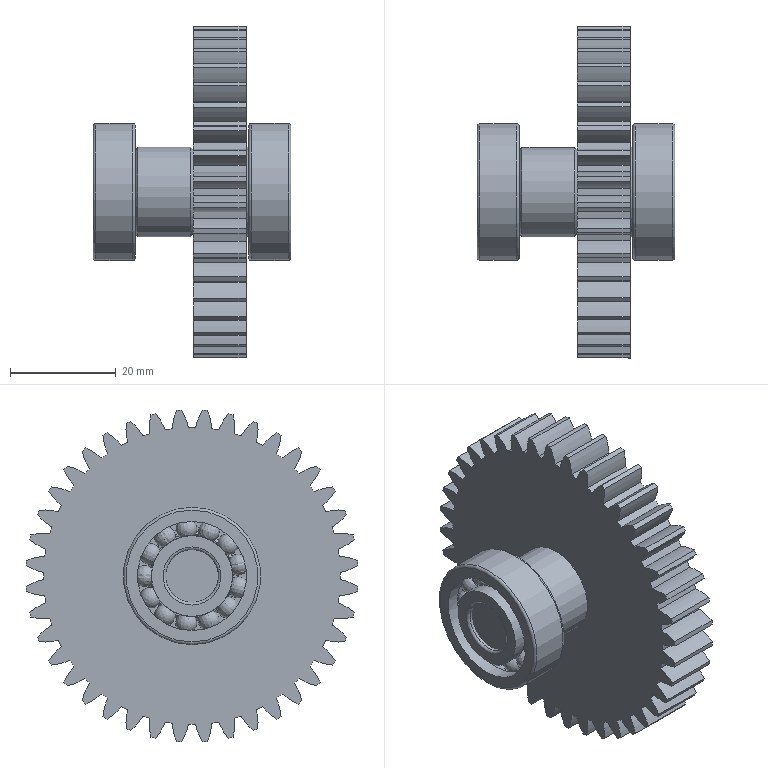Part | NX | features BREP 5 | 6 solids | 298 faces | box 37.5 x 62.872 x 62.872 mm | volume 37345 mm3 | cylinder 182 | torus 60 | plane 26 | sphere 26 | cone 4 | commonest cylinder face diameters 24 x80 56.248 x40 63 x40 4 x4 15.333 x4 20.667 x4